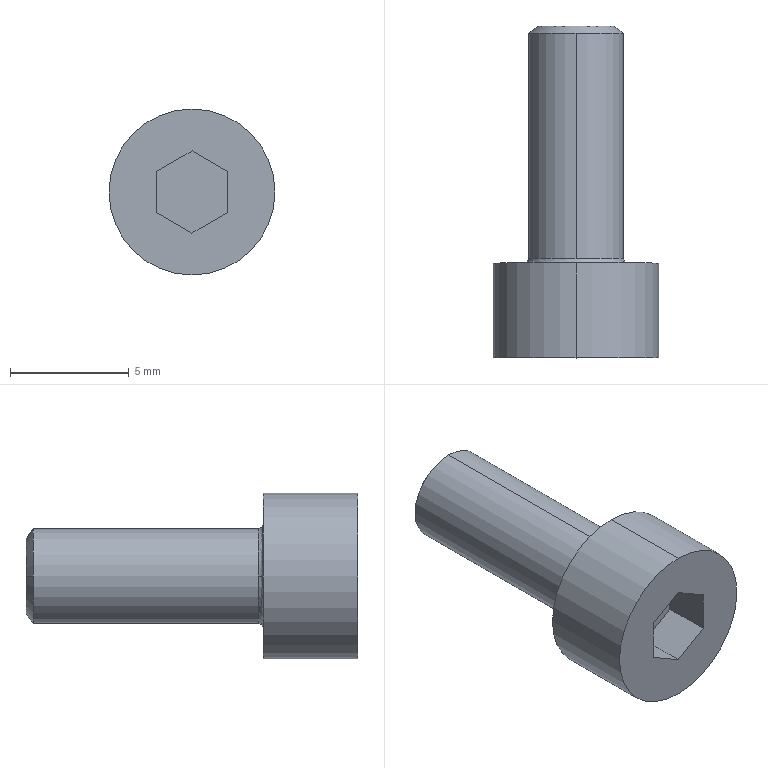Part | STEP file | 1 solid | 19 faces | box 7 x 14 x 7 mm | volume 263.372 mm3 | plane 10 | cylinder 4 | cone 3 | spline 2 | commonest cylinder face diameters 4 x2 7 x2